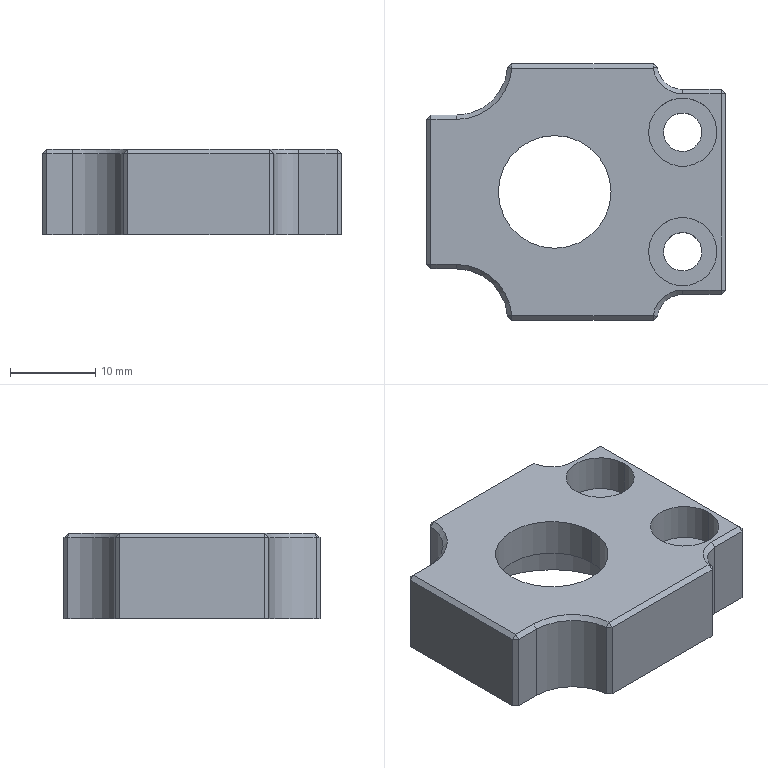Part | STEP file | 03-35 guide bushing mounting seat | 1 solid | 57 faces | box 35 x 30 x 10 mm | volume 5722 mm3 | plane 37 | cylinder 16 | cone 4 | commonest cylinder face diameters 4.5 x4 8 x4 6 x2 12 x2 13.2 x2 22 x2
STEP:
#1=CARTESIAN_POINT('',(8.5,7.,5.6));
#2=VERTEX_POINT('',#1);
#3=CARTESIAN_POINT('',(16.5,7.,5.6));
#4=VERTEX_POINT('',#3);
#5=CARTESIAN_POINT('',(12.5,7.,5.6));
#6=DIRECTION('',(0.,0.,1.));
#7=DIRECTION('',(1.,0.,0.));
#8=AXIS2_PLACEMENT_3D('',#5,#6,#7);
#9=CIRCLE('',#8,4.);
#10=EDGE_CURVE('',#2,#4,#9,.T.);
#11=ORIENTED_EDGE('',*,*,#10,.F.);
#12=CARTESIAN_POINT('',(8.5,7.,10.));
#13=VERTEX_POINT('',#12);
#14=CARTESIAN_POINT('',(8.5,7.,10.));
#15=DIRECTION('',(0.,0.,1.));
#16=VECTOR('',#15,1000.);
#17=LINE('',#14,#16);
#18=EDGE_CURVE('',#2,#13,#17,.T.);
#19=ORIENTED_EDGE('',*,*,#18,.T.);
#20=CARTESIAN_POINT('',(16.5,7.,10.));
#21=VERTEX_POINT('',#20);
#22=CARTESIAN_POINT('',(12.5,7.,10.));
#23=DIRECTION('',(0.,0.,1.));
#24=DIRECTION('',(1.,0.,0.));
#25=AXIS2_PLACEMENT_3D('',#22,#23,#24);
#26=CIRCLE('',#25,4.);
#27=EDGE_CURVE('',#13,#21,#26,.T.);
#28=ORIENTED_EDGE('',*,*,#27,.T.);
#29=CARTESIAN_POINT('',(16.5,7.,10.));
#30=DIRECTION('',(0.,0.,1.));
#31=VECTOR('',#30,1000.);
#32=LINE('',#29,#31);
#33=EDGE_CURVE('',#4,#21,#32,.T.);
#34=ORIENTED_EDGE('',*,*,#33,.F.);
#35=EDGE_LOOP('',(#11,#19,#28,#34));
#36=FACE_OUTER_BOUND('',#35,.T.);
#37=CARTESIAN_POINT('',(12.5,7.,10.));
#38=DIRECTION('',(0.,0.,1.));
#39=DIRECTION('',(1.,0.,0.));
#40=AXIS2_PLACEMENT_3D('',#37,#38,#39);
#41=CYLINDRICAL_SURFACE('',#40,4.);
#42=ADVANCED_FACE('',(#36),#41,.F.);
#43=CARTESIAN_POINT('',(10.25,7.,0.));
#44=VERTEX_POINT('',#43);
#45=CARTESIAN_POINT('',(14.75,7.,0.));
#46=VERTEX_POINT('',#45);
#47=CARTESIAN_POINT('',(12.5,7.,0.));
#48=DIRECTION('',(0.,0.,1.));
#49=DIRECTION('',(1.,0.,0.));
#50=AXIS2_PLACEMENT_3D('',#47,#48,#49);
#51=CIRCLE('',#50,2.25);
#52=EDGE_CURVE('',#44,#46,#51,.T.);
#53=ORIENTED_EDGE('',*,*,#52,.F.);
#54=CARTESIAN_POINT('',(10.25,7.,5.6));
#55=VERTEX_POINT('',#54);
#56=CARTESIAN_POINT('',(10.25,7.,10.));
#57=DIRECTION('',(0.,0.,1.));
#58=VECTOR('',#57,1000.);
#59=LINE('',#56,#58);
#60=EDGE_CURVE('',#44,#55,#59,.T.);
#61=ORIENTED_EDGE('',*,*,#60,.T.);
#62=CARTESIAN_POINT('',(14.75,7.,5.6));
#63=VERTEX_POINT('',#62);
#64=CARTESIAN_POINT('',(12.5,7.,5.6));
#65=DIRECTION('',(0.,0.,1.));
#66=DIRECTION('',(1.,0.,0.));
#67=AXIS2_PLACEMENT_3D('',#64,#65,#66);
#68=CIRCLE('',#67,2.25);
#69=EDGE_CURVE('',#55,#63,#68,.T.);
#70=ORIENTED_EDGE('',*,*,#69,.T.);
#71=CARTESIAN_POINT('',(14.75,7.,10.));
#72=DIRECTION('',(0.,0.,1.));
#73=VECTOR('',#72,1000.);
#74=LINE('',#71,#73);
#75=EDGE_CURVE('',#46,#63,#74,.T.);
#76=ORIENTED_EDGE('',*,*,#75,.F.);
#77=EDGE_LOOP('',(#53,#61,#70,#76));
#78=FACE_OUTER_BOUND('',#77,.T.);
#79=CARTESIAN_POINT('',(12.5,7.,10.));
#80=DIRECTION('',(0.,0.,1.));
#81=DIRECTION('',(1.,0.,0.));
#82=AXIS2_PLACEMENT_3D('',#79,#80,#81);
#83=CYLINDRICAL_SURFACE('',#82,2.25);
#84=ADVANCED_FACE('',(#78),#83,.F.);
#85=CARTESIAN_POINT('',(8.5,-7.,5.6));
#86=VERTEX_POINT('',#85);
#87=CARTESIAN_POINT('',(16.5,-7.,5.6));
#88=VERTEX_POINT('',#87);
#89=CARTESIAN_POINT('',(12.5,-7.,5.6));
#90=DIRECTION('',(0.,0.,1.));
#91=DIRECTION('',(1.,0.,0.));
#92=AXIS2_PLACEMENT_3D('',#89,#90,#91);
#93=CIRCLE('',#92,4.);
#94=EDGE_CURVE('',#86,#88,#93,.T.);
#95=ORIENTED_EDGE('',*,*,#94,.F.);
#96=CARTESIAN_POINT('',(8.5,-7.,10.));
#97=VERTEX_POINT('',#96);
#98=CARTESIAN_POINT('',(8.5,-7.,10.));
#99=DIRECTION('',(0.,0.,1.));
#100=VECTOR('',#99,1000.);
#101=LINE('',#98,#100);
#102=EDGE_CURVE('',#86,#97,#101,.T.);
#103=ORIENTED_EDGE('',*,*,#102,.T.);
#104=CARTESIAN_POINT('',(16.5,-7.,10.));
#105=VERTEX_POINT('',#104);
#106=CARTESIAN_POINT('',(12.5,-7.,10.));
#107=DIRECTION('',(0.,0.,1.));
#108=DIRECTION('',(1.,0.,0.));
#109=AXIS2_PLACEMENT_3D('',#106,#107,#108);
#110=CIRCLE('',#109,4.);
#111=EDGE_CURVE('',#97,#105,#110,.T.);
#112=ORIENTED_EDGE('',*,*,#111,.T.);
#113=CARTESIAN_POINT('',(16.5,-7.,10.));
#114=DIRECTION('',(0.,0.,1.));
#115=VECTOR('',#114,1000.);
#116=LINE('',#113,#115);
#117=EDGE_CURVE('',#88,#105,#116,.T.);
#118=ORIENTED_EDGE('',*,*,#117,.F.);
#119=EDGE_LOOP('',(#95,#103,#112,#118));
#120=FACE_OUTER_BOUND('',#119,.T.);
#121=CARTESIAN_POINT('',(12.5,-7.,10.));
#122=DIRECTION('',(0.,0.,1.));
#123=DIRECTION('',(1.,0.,0.));
#124=AXIS2_PLACEMENT_3D('',#121,#122,#123);
#125=CYLINDRICAL_SURFACE('',#124,4.);
#126=ADVANCED_FACE('',(#120),#125,.F.);
#127=CARTESIAN_POINT('',(10.25,-7.,0.));
#128=VERTEX_POINT('',#127);
#129=CARTESIAN_POINT('',(14.75,-7.,0.));
#130=VERTEX_POINT('',#129);
#131=CARTESIAN_POINT('',(12.5,-7.,0.));
#132=DIRECTION('',(0.,0.,1.));
#133=DIRECTION('',(1.,0.,0.));
#134=AXIS2_PLACEMENT_3D('',#131,#132,#133);
#135=CIRCLE('',#134,2.25);
#136=EDGE_CURVE('',#128,#130,#135,.T.);
#137=ORIENTED_EDGE('',*,*,#136,.F.);
#138=CARTESIAN_POINT('',(10.25,-7.,5.6));
#139=VERTEX_POINT('',#138);
#140=CARTESIAN_POINT('',(10.25,-7.,10.));
#141=DIRECTION('',(0.,0.,1.));
#142=VECTOR('',#141,1000.);
#143=LINE('',#140,#142);
#144=EDGE_CURVE('',#128,#139,#143,.T.);
#145=ORIENTED_EDGE('',*,*,#144,.T.);
#146=CARTESIAN_POINT('',(14.75,-7.,5.6));
#147=VERTEX_POINT('',#146);
#148=CARTESIAN_POINT('',(12.5,-7.,5.6));
#149=DIRECTION('',(0.,0.,1.));
#150=DIRECTION('',(1.,0.,0.));
#151=AXIS2_PLACEMENT_3D('',#148,#149,#150);
#152=CIRCLE('',#151,2.25);
#153=EDGE_CURVE('',#139,#147,#152,.T.);
#154=ORIENTED_EDGE('',*,*,#153,.T.);
#155=CARTESIAN_POINT('',(14.75,-7.,10.));
#156=DIRECTION('',(0.,0.,1.));
#157=VECTOR('',#156,1000.);
#158=LINE('',#155,#157);
#159=EDGE_CURVE('',#130,#147,#158,.T.);
#160=ORIENTED_EDGE('',*,*,#159,.F.);
#161=EDGE_LOOP('',(#137,#145,#154,#160));
#162=FACE_OUTER_BOUND('',#161,.T.);
#163=CARTESIAN_POINT('',(12.5,-7.,10.));
#164=DIRECTION('',(0.,0.,1.));
#165=DIRECTION('',(1.,0.,0.));
#166=AXIS2_PLACEMENT_3D('',#163,#164,#165);
#167=CYLINDRICAL_SURFACE('',#166,2.25);
#168=ADVANCED_FACE('',(#162),#167,.F.);
#169=CARTESIAN_POINT('',(8.5,0.,5.5));
#170=VERTEX_POINT('',#169);
#171=CARTESIAN_POINT('',(-13.5,0.,5.5));
#172=VERTEX_POINT('',#171);
#173=CARTESIAN_POINT('',(-2.5,0.,5.5));
#174=DIRECTION('',(0.,0.,-1.));
#175=DIRECTION('',(-1.,0.,0.));
#176=AXIS2_PLACEMENT_3D('',#173,#174,#175);
#177=CIRCLE('',#176,11.);
#178=EDGE_CURVE('',#170,#172,#177,.T.);
#179=ORIENTED_EDGE('',*,*,#178,.F.);
#180=CARTESIAN_POINT('',(8.5,0.,0.));
#181=VERTEX_POINT('',#180);
#182=CARTESIAN_POINT('',(8.5,0.,5.5));
#183=DIRECTION('',(0.,0.,-1.));
#184=VECTOR('',#183,1000.);
#185=LINE('',#182,#184);
#186=EDGE_CURVE('',#170,#181,#185,.T.);
#187=ORIENTED_EDGE('',*,*,#186,.T.);
#188=CARTESIAN_POINT('',(-13.5,0.,0.));
#189=VERTEX_POINT('',#188);
#190=CARTESIAN_POINT('',(-2.5,0.,0.));
#191=DIRECTION('',(0.,0.,-1.));
#192=DIRECTION('',(-1.,0.,0.));
#193=AXIS2_PLACEMENT_3D('',#190,#191,#192);
#194=CIRCLE('',#193,11.);
#195=EDGE_CURVE('',#181,#189,#194,.T.);
#196=ORIENTED_EDGE('',*,*,#195,.T.);
#197=CARTESIAN_POINT('',(-13.5,0.,5.5));
#198=DIRECTION('',(0.,0.,-1.));
#199=VECTOR('',#198,1000.);
#200=LINE('',#197,#199);
#201=EDGE_CURVE('',#172,#189,#200,.T.);
#202=ORIENTED_EDGE('',*,*,#201,.F.);
#203=EDGE_LOOP('',(#179,#187,#196,#202));
#204=FACE_OUTER_BOUND('',#203,.T.);
#205=CARTESIAN_POINT('',(-2.5,0.,5.5));
#206=DIRECTION('',(0.,0.,-1.));
#207=DIRECTION('',(-1.,0.,0.));
#208=AXIS2_PLACEMENT_3D('',#205,#206,#207);
#209=CYLINDRICAL_SURFACE('',#208,11.);
#210=ADVANCED_FACE('',(#204),#209,.F.);
#211=CARTESIAN_POINT('',(-9.1,0.,5.5));
#212=VERTEX_POINT('',#211);
#213=CARTESIAN_POINT('',(4.1,0.,5.5));
#214=VERTEX_POINT('',#213);
#215=CARTESIAN_POINT('',(-2.5,0.,5.5));
#216=DIRECTION('',(0.,0.,1.));
#217=DIRECTION('',(-1.,0.,0.));
#218=AXIS2_PLACEMENT_3D('',#215,#216,#217);
#219=CIRCLE('',#218,6.6);
#220=EDGE_CURVE('',#212,#214,#219,.T.);
#221=ORIENTED_EDGE('',*,*,#220,.F.);
#222=CARTESIAN_POINT('',(-9.1,0.,10.));
#223=VERTEX_POINT('',#222);
#224=CARTESIAN_POINT('',(-9.1,0.,-10.));
#225=DIRECTION('',(0.,0.,1.));
#226=VECTOR('',#225,1000.);
#227=LINE('',#224,#226);
#228=EDGE_CURVE('',#212,#223,#227,.T.);
#229=ORIENTED_EDGE('',*,*,#228,.T.);
#230=CARTESIAN_POINT('',(4.1,0.,10.));
#231=VERTEX_POINT('',#230);
#232=CARTESIAN_POINT('',(-2.5,0.,10.));
#233=DIRECTION('',(0.,0.,1.));
#234=DIRECTION('',(1.,0.,0.));
#235=AXIS2_PLACEMENT_3D('',#232,#233,#234);
#236=CIRCLE('',#235,6.6);
#237=EDGE_CURVE('',#223,#231,#236,.T.);
#238=ORIENTED_EDGE('',*,*,#237,.T.);
#239=CARTESIAN_POINT('',(4.1,0.,-10.));
#240=DIRECTION('',(0.,0.,1.));
#241=VECTOR('',#240,1000.);
#242=LINE('',#239,#241);
#243=EDGE_CURVE('',#214,#231,#242,.T.);
#244=ORIENTED_EDGE('',*,*,#243,.F.);
#245=EDGE_LOOP('',(#221,#229,#238,#244));
#246=FACE_OUTER_BOUND('',#245,.T.);
#247=CARTESIAN_POINT('',(-2.5,0.,-10.));
#248=DIRECTION('',(0.,0.,1.));
#249=DIRECTION('',(1.,0.,0.));
#250=AXIS2_PLACEMENT_3D('',#247,#248,#249);
#251=CYLINDRICAL_SURFACE('',#250,6.6);
#252=ADVANCED_FACE('',(#246),#251,.F.);
#253=ORIENTED_EDGE('',*,*,#228,.F.);
#254=CARTESIAN_POINT('',(-2.5,0.,5.5));
#255=DIRECTION('',(0.,0.,1.));
#256=DIRECTION('',(-1.,0.,0.));
#257=AXIS2_PLACEMENT_3D('',#254,#255,#256);
#258=CIRCLE('',#257,6.6);
#259=EDGE_CURVE('',#214,#212,#258,.T.);
#260=ORIENTED_EDGE('',*,*,#259,.F.);
#261=ORIENTED_EDGE('',*,*,#243,.T.);
#262=CARTESIAN_POINT('',(-2.5,0.,10.));
#263=DIRECTION('',(0.,0.,1.));
#264=DIRECTION('',(1.,0.,0.));
#265=AXIS2_PLACEMENT_3D('',#262,#263,#264);
#266=CIRCLE('',#265,6.6);
#267=EDGE_CURVE('',#231,#223,#266,.T.);
#268=ORIENTED_EDGE('',*,*,#267,.T.);
#269=EDGE_LOOP('',(#253,#260,#261,#268));
#270=FACE_OUTER_BOUND('',#269,.T.);
#271=CARTESIAN_POINT('',(-2.5,0.,-10.));
#272=DIRECTION('',(0.,0.,1.));
#273=DIRECTION('',(1.,0.,0.));
#274=AXIS2_PLACEMENT_3D('',#271,#272,#273);
#275=CYLINDRICAL_SURFACE('',#274,6.6);
#276=ADVANCED_FACE('',(#270),#275,.F.);
#277=CARTESIAN_POINT('',(17.5,11.5,9.5));
#278=VERTEX_POINT('',#277);
#279=CARTESIAN_POINT('',(17.5,-11.5,9.5));
#280=VERTEX_POINT('',#279);
#281=CARTESIAN_POINT('',(17.5,-12.,9.5));
#282=DIRECTION('',(0.,-1.,0.));
#283=VECTOR('',#282,1000.);
#284=LINE('',#281,#283);
#285=EDGE_CURVE('',#278,#280,#284,.T.);
#286=ORIENTED_EDGE('',*,*,#285,.T.);
#287=CARTESIAN_POINT('',(17.5,-11.5,0.));
#288=VERTEX_POINT('',#287);
#289=CARTESIAN_POINT('',(17.5,-11.5,10.));
#290=DIRECTION('',(0.,0.,-1.));
#291=VECTOR('',#290,1000.);
#292=LINE('',#289,#291);
#293=EDGE_CURVE('',#280,#288,#292,.T.);
#294=ORIENTED_EDGE('',*,*,#293,.T.);
#295=CARTESIAN_POINT('',(17.5,11.5,0.));
#296=VERTEX_POINT('',#295);
#297=CARTESIAN_POINT('',(17.5,15.,0.));
#298=DIRECTION('',(0.,1.,0.));
#299=VECTOR('',#298,1000.);
#300=LINE('',#297,#299);
#301=EDGE_CURVE('',#288,#296,#300,.T.);
#302=ORIENTED_EDGE('',*,*,#301,.T.);
#303=CARTESIAN_POINT('',(17.5,11.5,10.));
#304=DIRECTION('',(0.,0.,1.));
#305=VECTOR('',#304,1000.);
#306=LINE('',#303,#305);
#307=EDGE_CURVE('',#296,#278,#306,.T.);
#308=ORIENTED_EDGE('',*,*,#307,.T.);
#309=EDGE_LOOP('',(#286,#294,#302,#308));
#310=FACE_OUTER_BOUND('',#309,.T.);
#311=CARTESIAN_POINT('',(17.5,15.,10.));
#312=DIRECTION('',(-1.,0.,0.));
#313=DIRECTION('',(0.,-1.,0.));
#314=AXIS2_PLACEMENT_3D('',#311,#312,#313);
#315=PLANE('',#314);
#316=ADVANCED_FACE('',(#310),#315,.F.);
#317=CARTESIAN_POINT('',(-7.519,15.,9.5));
#318=VERTEX_POINT('',#317);
#319=CARTESIAN_POINT('',(9.036,15.,9.5));
#320=VERTEX_POINT('',#319);
#321=CARTESIAN_POINT('',(9.5,15.,9.5));
#322=DIRECTION('',(1.,0.,0.));
#323=VECTOR('',#322,1000.);
#324=LINE('',#321,#323);
#325=EDGE_CURVE('',#318,#320,#324,.T.);
#326=ORIENTED_EDGE('',*,*,#325,.T.);
#327=CARTESIAN_POINT('',(9.036,15.,0.));
#328=VERTEX_POINT('',#327);
#329=CARTESIAN_POINT('',(9.036,15.,10.));
#330=DIRECTION('',(0.,0.,-1.));
#331=VECTOR('',#330,1000.);
#332=LINE('',#329,#331);
#333=EDGE_CURVE('',#320,#328,#332,.T.);
#334=ORIENTED_EDGE('',*,*,#333,.T.);
#335=CARTESIAN_POINT('',(-7.519,15.,0.));
#336=VERTEX_POINT('',#335);
#337=CARTESIAN_POINT('',(-17.5,15.,0.));
#338=DIRECTION('',(-1.,0.,0.));
#339=VECTOR('',#338,1000.);
#340=LINE('',#337,#339);
#341=EDGE_CURVE('',#328,#336,#340,.T.);
#342=ORIENTED_EDGE('',*,*,#341,.T.);
#343=CARTESIAN_POINT('',(-7.519,15.,10.));
#344=DIRECTION('',(0.,0.,1.));
#345=VECTOR('',#344,1000.);
#346=LINE('',#343,#345);
#347=EDGE_CURVE('',#336,#318,#346,.T.);
#348=ORIENTED_EDGE('',*,*,#347,.T.);
#349=EDGE_LOOP('',(#326,#334,#342,#348));
#350=FACE_OUTER_BOUND('',#349,.T.);
#351=CARTESIAN_POINT('',(-17.5,15.,10.));
#352=DIRECTION('',(0.,-1.,0.));
#353=DIRECTION('',(0.,0.,-1.));
#354=AXIS2_PLACEMENT_3D('',#351,#352,#353);
#355=PLANE('',#354);
#356=ADVANCED_FACE('',(#350),#355,.F.);
#357=CARTESIAN_POINT('',(-17.5,-8.5,9.5));
#358=VERTEX_POINT('',#357);
#359=CARTESIAN_POINT('',(-17.5,8.5,9.5));
#360=VERTEX_POINT('',#359);
#361=CARTESIAN_POINT('',(-17.5,9.,9.5));
#362=DIRECTION('',(0.,1.,0.));
#363=VECTOR('',#362,1000.);
#364=LINE('',#361,#363);
#365=EDGE_CURVE('',#358,#360,#364,.T.);
#366=ORIENTED_EDGE('',*,*,#365,.T.);
#367=CARTESIAN_POINT('',(-17.5,8.5,0.));
#368=VERTEX_POINT('',#367);
#369=CARTESIAN_POINT('',(-17.5,8.5,10.));
#370=DIRECTION('',(0.,0.,-1.));
#371=VECTOR('',#370,1000.);
#372=LINE('',#369,#371);
#373=EDGE_CURVE('',#360,#368,#372,.T.);
#374=ORIENTED_EDGE('',*,*,#373,.T.);
#375=CARTESIAN_POINT('',(-17.5,-8.5,0.));
#376=VERTEX_POINT('',#375);
#377=CARTESIAN_POINT('',(-17.5,15.,0.));
#378=DIRECTION('',(0.,-1.,0.));
#379=VECTOR('',#378,1000.);
#380=LINE('',#377,#379);
#381=EDGE_CURVE('',#368,#376,#380,.T.);
#382=ORIENTED_EDGE('',*,*,#381,.T.);
#383=CARTESIAN_POINT('',(-17.5,-8.5,10.));
#384=DIRECTION('',(0.,0.,1.));
#385=VECTOR('',#384,1000.);
#386=LINE('',#383,#385);
#387=EDGE_CURVE('',#376,#358,#386,.T.);
#388=ORIENTED_EDGE('',*,*,#387,.T.);
#389=EDGE_LOOP('',(#366,#374,#382,#388));
#390=FACE_OUTER_BOUND('',#389,.T.);
#391=CARTESIAN_POINT('',(-17.5,15.,10.));
#392=DIRECTION('',(1.,0.,0.));
#393=DIRECTION('',(0.,1.,0.));
#394=AXIS2_PLACEMENT_3D('',#391,#392,#393);
#395=PLANE('',#394);
#396=ADVANCED_FACE('',(#390),#395,.F.);
#397=CARTESIAN_POINT('',(9.036,-15.,9.5));
#398=VERTEX_POINT('',#397);
#399=CARTESIAN_POINT('',(-7.519,-15.,9.5));
#400=VERTEX_POINT('',#399);
#401=CARTESIAN_POINT('',(-8.,-15.,9.5));
#402=DIRECTION('',(-1.,0.,0.));
#403=VECTOR('',#402,1000.);
#404=LINE('',#401,#403);
#405=EDGE_CURVE('',#398,#400,#404,.T.);
#406=ORIENTED_EDGE('',*,*,#405,.T.);
#407=CARTESIAN_POINT('',(-7.519,-15.,0.));
#408=VERTEX_POINT('',#407);
#409=CARTESIAN_POINT('',(-7.519,-15.,10.));
#410=DIRECTION('',(0.,0.,-1.));
#411=VECTOR('',#410,1000.);
#412=LINE('',#409,#411);
#413=EDGE_CURVE('',#400,#408,#412,.T.);
#414=ORIENTED_EDGE('',*,*,#413,.T.);
#415=CARTESIAN_POINT('',(9.036,-15.,0.));
#416=VERTEX_POINT('',#415);
#417=CARTESIAN_POINT('',(-17.5,-15.,0.));
#418=DIRECTION('',(1.,0.,0.));
#419=VECTOR('',#418,1000.);
#420=LINE('',#417,#419);
#421=EDGE_CURVE('',#408,#416,#420,.T.);
#422=ORIENTED_EDGE('',*,*,#421,.T.);
#423=CARTESIAN_POINT('',(9.036,-15.,10.));
#424=DIRECTION('',(0.,0.,1.));
#425=VECTOR('',#424,1000.);
#426=LINE('',#423,#425);
#427=EDGE_CURVE('',#416,#398,#426,.T.);
#428=ORIENTED_EDGE('',*,*,#427,.T.);
#429=EDGE_LOOP('',(#406,#414,#422,#428));
#430=FACE_OUTER_BOUND('',#429,.T.);
#431=CARTESIAN_POINT('',(-17.5,-15.,10.));
#432=DIRECTION('',(0.,1.,0.));
#433=DIRECTION('',(0.,0.,1.));
#434=AXIS2_PLACEMENT_3D('',#431,#432,#433);
#435=PLANE('',#434);
#436=ADVANCED_FACE('',(#430),#435,.F.);
#437=CARTESIAN_POINT('',(12.5,-11.5,10.));
#438=VERTEX_POINT('',#437);
#439=CARTESIAN_POINT('',(17.,-11.5,10.));
#440=VERTEX_POINT('',#439);
#441=CARTESIAN_POINT('',(17.5,-11.5,10.));
#442=DIRECTION('',(1.,0.,0.));
#443=VECTOR('',#442,1000.);
#444=LINE('',#441,#443);
#445=EDGE_CURVE('',#438,#440,#444,.T.);
#446=ORIENTED_EDGE('',*,*,#445,.T.);
#447=CARTESIAN_POINT('',(17.,11.5,10.));
#448=VERTEX_POINT('',#447);
#449=CARTESIAN_POINT('',(17.,12.,10.));
#450=DIRECTION('',(0.,1.,0.));
#451=VECTOR('',#450,1000.);
#452=LINE('',#449,#451);
#453=EDGE_CURVE('',#440,#448,#452,.T.);
#454=ORIENTED_EDGE('',*,*,#453,.T.);
#455=CARTESIAN_POINT('',(12.5,11.5,10.));
#456=VERTEX_POINT('',#455);
#457=CARTESIAN_POINT('',(12.5,11.5,10.));
#458=DIRECTION('',(-1.,0.,0.));
#459=VECTOR('',#458,1000.);
#460=LINE('',#457,#459);
#461=EDGE_CURVE('',#448,#456,#460,.T.);
#462=ORIENTED_EDGE('',*,*,#461,.T.);
#463=CARTESIAN_POINT('',(9.036,14.5,10.));
#464=VERTEX_POINT('',#463);
#465=CARTESIAN_POINT('',(12.5,15.,10.));
#466=DIRECTION('',(0.,0.,-1.));
#467=DIRECTION('',(1.,0.,0.));
#468=AXIS2_PLACEMENT_3D('',#465,#466,#467);
#469=CIRCLE('',#468,3.5);
#470=EDGE_CURVE('',#456,#464,#469,.T.);
#471=ORIENTED_EDGE('',*,*,#470,.T.);
#472=CARTESIAN_POINT('',(-7.519,14.5,10.));
#473=VERTEX_POINT('',#472);
#474=CARTESIAN_POINT('',(-8.,14.5,10.));
#475=DIRECTION('',(-1.,0.,0.));
#476=VECTOR('',#475,1000.);
#477=LINE('',#474,#476);
#478=EDGE_CURVE('',#464,#473,#477,.T.);
#479=ORIENTED_EDGE('',*,*,#478,.T.);
#480=CARTESIAN_POINT('',(-14.,8.5,10.));
#481=VERTEX_POINT('',#480);
#482=CARTESIAN_POINT('',(-14.,15.,10.));
#483=DIRECTION('',(0.,0.,-1.));
#484=DIRECTION('',(1.,0.,0.));
#485=AXIS2_PLACEMENT_3D('',#482,#483,#484);
#486=CIRCLE('',#485,6.5);
#487=EDGE_CURVE('',#473,#481,#486,.T.);
#488=ORIENTED_EDGE('',*,*,#487,.T.);
#489=CARTESIAN_POINT('',(-17.,8.5,10.));
#490=VERTEX_POINT('',#489);
#491=CARTESIAN_POINT('',(-17.5,8.5,10.));
#492=DIRECTION('',(-1.,0.,0.));
#493=VECTOR('',#492,1000.);
#494=LINE('',#491,#493);
#495=EDGE_CURVE('',#481,#490,#494,.T.);
#496=ORIENTED_EDGE('',*,*,#495,.T.);
#497=CARTESIAN_POINT('',(-17.,-8.5,10.));
#498=VERTEX_POINT('',#497);
#499=CARTESIAN_POINT('',(-17.,-9.,10.));
#500=DIRECTION('',(0.,-1.,0.));
#501=VECTOR('',#500,1000.);
#502=LINE('',#499,#501);
#503=EDGE_CURVE('',#490,#498,#502,.T.);
#504=ORIENTED_EDGE('',*,*,#503,.T.);
#505=CARTESIAN_POINT('',(-14.,-8.5,10.));
#506=VERTEX_POINT('',#505);
#507=CARTESIAN_POINT('',(-14.,-8.5,10.));
#508=DIRECTION('',(1.,0.,0.));
#509=VECTOR('',#508,1000.);
#510=LINE('',#507,#509);
#511=EDGE_CURVE('',#498,#506,#510,.T.);
#512=ORIENTED_EDGE('',*,*,#511,.T.);
#513=CARTESIAN_POINT('',(-7.519,-14.5,10.));
#514=VERTEX_POINT('',#513);
#515=CARTESIAN_POINT('',(-14.,-15.,10.));
#516=DIRECTION('',(0.,0.,-1.));
#517=DIRECTION('',(1.,0.,0.));
#518=AXIS2_PLACEMENT_3D('',#515,#516,#517);
#519=CIRCLE('',#518,6.5);
#520=EDGE_CURVE('',#506,#514,#519,.T.);
#521=ORIENTED_EDGE('',*,*,#520,.T.);
#522=CARTESIAN_POINT('',(9.036,-14.5,10.));
#523=VERTEX_POINT('',#522);
#524=CARTESIAN_POINT('',(9.5,-14.5,10.));
#525=DIRECTION('',(1.,0.,0.));
#526=VECTOR('',#525,1000.);
#527=LINE('',#524,#526);
#528=EDGE_CURVE('',#514,#523,#527,.T.);
#529=ORIENTED_EDGE('',*,*,#528,.T.);
#530=CARTESIAN_POINT('',(12.5,-15.,10.));
#531=DIRECTION('',(0.,0.,-1.));
#532=DIRECTION('',(1.,0.,0.));
#533=AXIS2_PLACEMENT_3D('',#530,#531,#532);
#534=CIRCLE('',#533,3.5);
#535=EDGE_CURVE('',#523,#438,#534,.T.);
#536=ORIENTED_EDGE('',*,*,#535,.T.);
#537=EDGE_LOOP('',(#446,#454,#462,#471,#479,#488,#496,#504,#512,#521,#529,#536));
#538=FACE_OUTER_BOUND('',#537,.T.);
#539=CARTESIAN_POINT('',(12.5,7.,10.));
#540=DIRECTION('',(0.,0.,1.));
#541=DIRECTION('',(1.,0.,0.));
#542=AXIS2_PLACEMENT_3D('',#539,#540,#541);
#543=CIRCLE('',#542,4.);
#544=EDGE_CURVE('',#21,#13,#543,.T.);
#545=ORIENTED_EDGE('',*,*,#544,.F.);
#546=ORIENTED_EDGE('',*,*,#27,.F.);
#547=EDGE_LOOP('',(#545,#546));
#548=FACE_BOUND('',#547,.T.);
#549=CARTESIAN_POINT('',(12.5,-7.,10.));
#550=DIRECTION('',(0.,0.,1.));
#551=DIRECTION('',(1.,0.,0.));
#552=AXIS2_PLACEMENT_3D('',#549,#550,#551);
#553=CIRCLE('',#552,4.);
#554=EDGE_CURVE('',#105,#97,#553,.T.);
#555=ORIENTED_EDGE('',*,*,#554,.F.);
#556=ORIENTED_EDGE('',*,*,#111,.F.);
#557=EDGE_LOOP('',(#555,#556));
#558=FACE_BOUND('',#557,.T.);
#559=ORIENTED_EDGE('',*,*,#267,.F.);
#560=ORIENTED_EDGE('',*,*,#237,.F.);
#561=EDGE_LOOP('',(#559,#560));
#562=FACE_BOUND('',#561,.T.);
#563=CARTESIAN_POINT('',(17.5,-15.,10.));
#564=DIRECTION('',(0.,0.,1.));
#565=DIRECTION('',(1.,0.,0.));
#566=AXIS2_PLACEMENT_3D('',#563,#564,#565);
#567=PLANE('',#566);
#568=ADVANCED_FACE('',(#538,#548,#558,#562),#567,.T.);
#569=CARTESIAN_POINT('',(12.5,7.,0.));
#570=DIRECTION('',(0.,0.,1.));
#571=DIRECTION('',(1.,0.,0.));
#572=AXIS2_PLACEMENT_3D('',#569,#570,#571);
#573=CIRCLE('',#572,2.25);
#574=EDGE_CURVE('',#46,#44,#573,.T.);
#575=ORIENTED_EDGE('',*,*,#574,.T.);
#576=ORIENTED_EDGE('',*,*,#52,.T.);
#577=EDGE_LOOP('',(#575,#576));
#578=FACE_BOUND('',#577,.T.);
#579=CARTESIAN_POINT('',(12.5,-7.,0.));
#580=DIRECTION('',(0.,0.,1.));
#581=DIRECTION('',(1.,0.,0.));
#582=AXIS2_PLACEMENT_3D('',#579,#580,#581);
#583=CIRCLE('',#582,2.25);
#584=EDGE_CURVE('',#130,#128,#583,.T.);
#585=ORIENTED_EDGE('',*,*,#584,.T.);
#586=ORIENTED_EDGE('',*,*,#136,.T.);
#587=EDGE_LOOP('',(#585,#586));
#588=FACE_BOUND('',#587,.T.);
#589=CARTESIAN_POINT('',(-2.5,0.,0.));
#590=DIRECTION('',(0.,0.,-1.));
#591=DIRECTION('',(-1.,0.,0.));
#592=AXIS2_PLACEMENT_3D('',#589,#590,#591);
#593=CIRCLE('',#592,11.);
#594=EDGE_CURVE('',#189,#181,#593,.T.);
#595=ORIENTED_EDGE('',*,*,#594,.F.);
#596=ORIENTED_EDGE('',*,*,#195,.F.);
#597=EDGE_LOOP('',(#595,#596));
#598=FACE_BOUND('',#597,.T.);
#599=ORIENTED_EDGE('',*,*,#301,.F.);
#600=CARTESIAN_POINT('',(17.,-12.,0.));
#601=VERTEX_POINT('',#600);
#602=CARTESIAN_POINT('',(17.,-12.,0.));
#603=DIRECTION('',(-0.7071,-0.7071,0.));
#604=VECTOR('',#603,1000.);
#605=LINE('',#602,#604);
#606=EDGE_CURVE('',#288,#601,#605,.T.);
#607=ORIENTED_EDGE('',*,*,#606,.T.);
#608=CARTESIAN_POINT('',(12.5,-12.,0.));
#609=VERTEX_POINT('',#608);
#610=CARTESIAN_POINT('',(17.5,-12.,0.));
#611=DIRECTION('',(-1.,0.,0.));
#612=VECTOR('',#611,1000.);
#613=LINE('',#610,#612);
#614=EDGE_CURVE('',#601,#609,#613,.T.);
#615=ORIENTED_EDGE('',*,*,#614,.T.);
#616=CARTESIAN_POINT('',(9.531,-14.571,0.));
#617=VERTEX_POINT('',#616);
#618=CARTESIAN_POINT('',(12.5,-15.,0.));
#619=DIRECTION('',(0.,0.,1.));
#620=DIRECTION('',(1.,0.,0.));
#621=AXIS2_PLACEMENT_3D('',#618,#619,#620);
#622=CIRCLE('',#621,3.);
#623=EDGE_CURVE('',#609,#617,#622,.T.);
#624=ORIENTED_EDGE('',*,*,#623,.T.);
#625=CARTESIAN_POINT('',(9.036,-15.,0.));
#626=DIRECTION('',(-0.7559,-0.6547,0.));
#627=VECTOR('',#626,1000.);
#628=LINE('',#625,#627);
#629=EDGE_CURVE('',#617,#416,#628,.T.);
#630=ORIENTED_EDGE('',*,*,#629,.T.);
#631=ORIENTED_EDGE('',*,*,#421,.F.);
#632=CARTESIAN_POINT('',(-8.018,-14.538,0.));
#633=VERTEX_POINT('',#632);
#634=CARTESIAN_POINT('',(-8.018,-14.538,0.));
#635=DIRECTION('',(-0.7338,0.6794,0.));
#636=VECTOR('',#635,1000.);
#637=LINE('',#634,#636);
#638=EDGE_CURVE('',#408,#633,#637,.T.);
#639=ORIENTED_EDGE('',*,*,#638,.T.);
#640=CARTESIAN_POINT('',(-14.,-9.,0.));
#641=VERTEX_POINT('',#640);
#642=CARTESIAN_POINT('',(-14.,-15.,0.));
#643=DIRECTION('',(0.,0.,1.));
#644=DIRECTION('',(1.,0.,0.));
#645=AXIS2_PLACEMENT_3D('',#642,#643,#644);
#646=CIRCLE('',#645,6.);
#647=EDGE_CURVE('',#633,#641,#646,.T.);
#648=ORIENTED_EDGE('',*,*,#647,.T.);
#649=CARTESIAN_POINT('',(-17.,-9.,0.));
#650=VERTEX_POINT('',#649);
#651=CARTESIAN_POINT('',(17.5,-9.,0.));
#652=DIRECTION('',(-1.,0.,0.));
#653=VECTOR('',#652,1000.);
#654=LINE('',#651,#653);
#655=EDGE_CURVE('',#641,#650,#654,.T.);
#656=ORIENTED_EDGE('',*,*,#655,.T.);
#657=CARTESIAN_POINT('',(-17.5,-8.5,0.));
#658=DIRECTION('',(-0.7071,0.7071,0.));
#659=VECTOR('',#658,1000.);
#660=LINE('',#657,#659);
#661=EDGE_CURVE('',#650,#376,#660,.T.);
#662=ORIENTED_EDGE('',*,*,#661,.T.);
#663=ORIENTED_EDGE('',*,*,#381,.F.);
#664=CARTESIAN_POINT('',(-17.,9.,0.));
#665=VERTEX_POINT('',#664);
#666=CARTESIAN_POINT('',(-17.5,8.5,0.));
#667=DIRECTION('',(0.7071,0.7071,0.));
#668=VECTOR('',#667,1000.);
#669=LINE('',#666,#668);
#670=EDGE_CURVE('',#368,#665,#669,.T.);
#671=ORIENTED_EDGE('',*,*,#670,.T.);
#672=CARTESIAN_POINT('',(-14.,9.,0.));
#673=VERTEX_POINT('',#672);
#674=CARTESIAN_POINT('',(17.5,9.,0.));
#675=DIRECTION('',(1.,0.,0.));
#676=VECTOR('',#675,1000.);
#677=LINE('',#674,#676);
#678=EDGE_CURVE('',#665,#673,#677,.T.);
#679=ORIENTED_EDGE('',*,*,#678,.T.);
#680=CARTESIAN_POINT('',(-8.018,14.538,0.));
#681=VERTEX_POINT('',#680);
#682=CARTESIAN_POINT('',(-14.,15.,0.));
#683=DIRECTION('',(0.,0.,1.));
#684=DIRECTION('',(1.,0.,0.));
#685=AXIS2_PLACEMENT_3D('',#682,#683,#684);
#686=CIRCLE('',#685,6.);
#687=EDGE_CURVE('',#673,#681,#686,.T.);
#688=ORIENTED_EDGE('',*,*,#687,.T.);
#689=CARTESIAN_POINT('',(-7.519,15.,0.));
#690=DIRECTION('',(0.7338,0.6794,0.));
#691=VECTOR('',#690,1000.);
#692=LINE('',#689,#691);
#693=EDGE_CURVE('',#681,#336,#692,.T.);
#694=ORIENTED_EDGE('',*,*,#693,.T.);
#695=ORIENTED_EDGE('',*,*,#341,.F.);
#696=CARTESIAN_POINT('',(9.531,14.571,0.));
#697=VERTEX_POINT('',#696);
#698=CARTESIAN_POINT('',(9.531,14.571,0.));
#699=DIRECTION('',(0.7559,-0.6547,0.));
#700=VECTOR('',#699,1000.);
#701=LINE('',#698,#700);
#702=EDGE_CURVE('',#328,#697,#701,.T.);
#703=ORIENTED_EDGE('',*,*,#702,.T.);
#704=CARTESIAN_POINT('',(12.5,12.,0.));
#705=VERTEX_POINT('',#704);
#706=CARTESIAN_POINT('',(12.5,15.,0.));
#707=DIRECTION('',(0.,0.,1.));
#708=DIRECTION('',(1.,0.,0.));
#709=AXIS2_PLACEMENT_3D('',#706,#707,#708);
#710=CIRCLE('',#709,3.);
#711=EDGE_CURVE('',#697,#705,#710,.T.);
#712=ORIENTED_EDGE('',*,*,#711,.T.);
#713=CARTESIAN_POINT('',(17.,12.,0.));
#714=VERTEX_POINT('',#713);
#715=CARTESIAN_POINT('',(17.5,12.,0.));
#716=DIRECTION('',(1.,0.,0.));
#717=VECTOR('',#716,1000.);
#718=LINE('',#715,#717);
#719=EDGE_CURVE('',#705,#714,#718,.T.);
#720=ORIENTED_EDGE('',*,*,#719,.T.);
#721=CARTESIAN_POINT('',(17.5,11.5,0.));
#722=DIRECTION('',(0.7071,-0.7071,0.));
#723=VECTOR('',#722,1000.);
#724=LINE('',#721,#723);
#725=EDGE_CURVE('',#714,#296,#724,.T.);
#726=ORIENTED_EDGE('',*,*,#725,.T.);
#727=EDGE_LOOP('',(#599,#607,#615,#624,#630,#631,#639,#648,#656,#662,#663,#671,#679,#688,#694,#695,#703,#712,#720,#726));
#728=FACE_OUTER_BOUND('',#727,.T.);
#729=CARTESIAN_POINT('',(17.5,-15.,0.));
#730=DIRECTION('',(0.,0.,1.));
#731=DIRECTION('',(1.,0.,0.));
#732=AXIS2_PLACEMENT_3D('',#729,#730,#731);
#733=PLANE('',#732);
#734=ADVANCED_FACE('',(#578,#588,#598,#728),#733,.F.);
#735=CARTESIAN_POINT('',(-14.,-9.,9.5));
#736=VERTEX_POINT('',#735);
#737=CARTESIAN_POINT('',(-17.,-9.,9.5));
#738=VERTEX_POINT('',#737);
#739=CARTESIAN_POINT('',(-17.5,-9.,9.5));
#740=DIRECTION('',(-1.,0.,0.));
#741=VECTOR('',#740,1000.);
#742=LINE('',#739,#741);
#743=EDGE_CURVE('',#736,#738,#742,.T.);
#744=ORIENTED_EDGE('',*,*,#743,.T.);
#745=CARTESIAN_POINT('',(-17.,-9.,-10.));
#746=DIRECTION('',(0.,0.,-1.));
#747=VECTOR('',#746,1000.);
#748=LINE('',#745,#747);
#749=EDGE_CURVE('',#738,#650,#748,.T.);
#750=ORIENTED_EDGE('',*,*,#749,.T.);
#751=ORIENTED_EDGE('',*,*,#655,.F.);
#752=CARTESIAN_POINT('',(-14.,-9.,10.));
#753=DIRECTION('',(0.,0.,1.));
#754=VECTOR('',#753,1000.);
#755=LINE('',#752,#754);
#756=EDGE_CURVE('',#641,#736,#755,.T.);
#757=ORIENTED_EDGE('',*,*,#756,.T.);
#758=EDGE_LOOP('',(#744,#750,#751,#757));
#759=FACE_OUTER_BOUND('',#758,.T.);
#760=CARTESIAN_POINT('',(-20.,-9.,-10.));
#761=DIRECTION('',(0.,1.,0.));
#762=DIRECTION('',(0.,0.,1.));
#763=AXIS2_PLACEMENT_3D('',#760,#761,#762);
#764=PLANE('',#763);
#765=ADVANCED_FACE('',(#759),#764,.F.);
#766=CARTESIAN_POINT('',(-17.,9.,9.5));
#767=VERTEX_POINT('',#766);
#768=CARTESIAN_POINT('',(-17.,9.,-10.));
#769=DIRECTION('',(0.,0.,1.));
#770=VECTOR('',#769,1000.);
#771=LINE('',#768,#770);
#772=EDGE_CURVE('',#665,#767,#771,.T.);
#773=ORIENTED_EDGE('',*,*,#772,.T.);
#774=CARTESIAN_POINT('',(-14.,9.,9.5));
#775=VERTEX_POINT('',#774);
#776=CARTESIAN_POINT('',(-14.,9.,9.5));
#777=DIRECTION('',(1.,0.,0.));
#778=VECTOR('',#777,1000.);
#779=LINE('',#776,#778);
#780=EDGE_CURVE('',#767,#775,#779,.T.);
#781=ORIENTED_EDGE('',*,*,#780,.T.);
#782=CARTESIAN_POINT('',(-14.,9.,5.5));
#783=DIRECTION('',(0.,0.,-1.));
#784=VECTOR('',#783,1000.);
#785=LINE('',#782,#784);
#786=EDGE_CURVE('',#775,#673,#785,.T.);
#787=ORIENTED_EDGE('',*,*,#786,.T.);
#788=ORIENTED_EDGE('',*,*,#678,.F.);
#789=EDGE_LOOP('',(#773,#781,#787,#788));
#790=FACE_OUTER_BOUND('',#789,.T.);
#791=CARTESIAN_POINT('',(-20.,9.,-10.));
#792=DIRECTION('',(0.,-1.,0.));
#793=DIRECTION('',(0.,0.,-1.));
#794=AXIS2_PLACEMENT_3D('',#791,#792,#793);
#795=PLANE('',#794);
#796=ADVANCED_FACE('',(#790),#795,.F.);
#797=ORIENTED_EDGE('',*,*,#186,.F.);
#798=CARTESIAN_POINT('',(-2.5,0.,5.5));
#799=DIRECTION('',(0.,0.,-1.));
#800=DIRECTION('',(-1.,0.,0.));
#801=AXIS2_PLACEMENT_3D('',#798,#799,#800);
#802=CIRCLE('',#801,11.);
#803=EDGE_CURVE('',#172,#170,#802,.T.);
#804=ORIENTED_EDGE('',*,*,#803,.F.);
#805=ORIENTED_EDGE('',*,*,#201,.T.);
#806=ORIENTED_EDGE('',*,*,#594,.T.);
#807=EDGE_LOOP('',(#797,#804,#805,#806));
#808=FACE_OUTER_BOUND('',#807,.T.);
#809=CARTESIAN_POINT('',(-2.5,0.,5.5));
#810=DIRECTION('',(0.,0.,-1.));
#811=DIRECTION('',(-1.,0.,0.));
#812=AXIS2_PLACEMENT_3D('',#809,#810,#811);
#813=CYLINDRICAL_SURFACE('',#812,11.);
#814=ADVANCED_FACE('',(#808),#813,.F.);
#815=ORIENTED_EDGE('',*,*,#259,.T.);
#816=ORIENTED_EDGE('',*,*,#220,.T.);
#817=EDGE_LOOP('',(#815,#816));
#818=FACE_BOUND('',#817,.T.);
#819=ORIENTED_EDGE('',*,*,#803,.T.);
#820=ORIENTED_EDGE('',*,*,#178,.T.);
#821=EDGE_LOOP('',(#819,#820));
#822=FACE_OUTER_BOUND('',#821,.T.);
#823=CARTESIAN_POINT('',(-2.5,0.,5.5));
#824=DIRECTION('',(0.,0.,-1.));
#825=DIRECTION('',(-1.,0.,0.));
#826=AXIS2_PLACEMENT_3D('',#823,#824,#825);
#827=PLANE('',#826);
#828=ADVANCED_FACE('',(#818,#822),#827,.T.);
#829=ORIENTED_EDGE('',*,*,#647,.F.);
#830=CARTESIAN_POINT('',(-8.018,-14.538,9.5));
#831=VERTEX_POINT('',#830);
#832=CARTESIAN_POINT('',(-8.018,-14.538,-10.));
#833=DIRECTION('',(0.,0.,1.));
#834=VECTOR('',#833,1000.);
#835=LINE('',#832,#834);
#836=EDGE_CURVE('',#633,#831,#835,.T.);
#837=ORIENTED_EDGE('',*,*,#836,.T.);
#838=CARTESIAN_POINT('',(-14.,-15.,9.5));
#839=DIRECTION('',(0.,0.,1.));
#840=DIRECTION('',(1.,0.,0.));
#841=AXIS2_PLACEMENT_3D('',#838,#839,#840);
#842=CIRCLE('',#841,6.);
#843=EDGE_CURVE('',#831,#736,#842,.T.);
#844=ORIENTED_EDGE('',*,*,#843,.T.);
#845=ORIENTED_EDGE('',*,*,#756,.F.);
#846=EDGE_LOOP('',(#829,#837,#844,#845));
#847=FACE_OUTER_BOUND('',#846,.T.);
#848=CARTESIAN_POINT('',(-14.,-15.,-10.));
#849=DIRECTION('',(0.,0.,-1.));
#850=DIRECTION('',(-1.,0.,0.));
#851=AXIS2_PLACEMENT_3D('',#848,#849,#850);
#852=CYLINDRICAL_SURFACE('',#851,6.);
#853=ADVANCED_FACE('',(#847),#852,.F.);
#854=CARTESIAN_POINT('',(-8.018,14.538,9.5));
#855=VERTEX_POINT('',#854);
#856=CARTESIAN_POINT('',(-14.,15.,9.5));
#857=DIRECTION('',(0.,0.,1.));
#858=DIRECTION('',(1.,0.,0.));
#859=AXIS2_PLACEMENT_3D('',#856,#857,#858);
#860=CIRCLE('',#859,6.);
#861=EDGE_CURVE('',#775,#855,#860,.T.);
#862=ORIENTED_EDGE('',*,*,#861,.T.);
#863=CARTESIAN_POINT('',(-8.018,14.538,-10.));
#864=DIRECTION('',(0.,0.,-1.));
#865=VECTOR('',#864,1000.);
#866=LINE('',#863,#865);
#867=EDGE_CURVE('',#855,#681,#866,.T.);
#868=ORIENTED_EDGE('',*,*,#867,.T.);
#869=ORIENTED_EDGE('',*,*,#687,.F.);
#870=ORIENTED_EDGE('',*,*,#786,.F.);
#871=EDGE_LOOP('',(#862,#868,#869,#870));
#872=FACE_OUTER_BOUND('',#871,.T.);
#873=CARTESIAN_POINT('',(-14.,15.,-10.));
#874=DIRECTION('',(0.,0.,-1.));
#875=DIRECTION('',(-1.,0.,0.));
#876=AXIS2_PLACEMENT_3D('',#873,#874,#875);
#877=CYLINDRICAL_SURFACE('',#876,6.);
#878=ADVANCED_FACE('',(#872),#877,.F.);
#879=ORIENTED_EDGE('',*,*,#144,.F.);
#880=ORIENTED_EDGE('',*,*,#584,.F.);
#881=ORIENTED_EDGE('',*,*,#159,.T.);
#882=CARTESIAN_POINT('',(12.5,-7.,5.6));
#883=DIRECTION('',(0.,0.,1.));
#884=DIRECTION('',(1.,0.,0.));
#885=AXIS2_PLACEMENT_3D('',#882,#883,#884);
#886=CIRCLE('',#885,2.25);
#887=EDGE_CURVE('',#147,#139,#886,.T.);
#888=ORIENTED_EDGE('',*,*,#887,.T.);
#889=EDGE_LOOP('',(#879,#880,#881,#888));
#890=FACE_OUTER_BOUND('',#889,.T.);
#891=CARTESIAN_POINT('',(12.5,-7.,10.));
#892=DIRECTION('',(0.,0.,1.));
#893=DIRECTION('',(1.,0.,0.));
#894=AXIS2_PLACEMENT_3D('',#891,#892,#893);
#895=CYLINDRICAL_SURFACE('',#894,2.25);
#896=ADVANCED_FACE('',(#890),#895,.F.);
#897=ORIENTED_EDGE('',*,*,#887,.F.);
#898=ORIENTED_EDGE('',*,*,#153,.F.);
#899=EDGE_LOOP('',(#897,#898));
#900=FACE_BOUND('',#899,.T.);
#901=CARTESIAN_POINT('',(12.5,-7.,5.6));
#902=DIRECTION('',(0.,0.,1.));
#903=DIRECTION('',(1.,0.,0.));
#904=AXIS2_PLACEMENT_3D('',#901,#902,#903);
#905=CIRCLE('',#904,4.);
#906=EDGE_CURVE('',#88,#86,#905,.T.);
#907=ORIENTED_EDGE('',*,*,#906,.T.);
#908=ORIENTED_EDGE('',*,*,#94,.T.);
#909=EDGE_LOOP('',(#907,#908));
#910=FACE_OUTER_BOUND('',#909,.T.);
#911=CARTESIAN_POINT('',(14.75,-7.,5.6));
#912=DIRECTION('',(0.,0.,-1.));
#913=DIRECTION('',(-1.,0.,0.));
#914=AXIS2_PLACEMENT_3D('',#911,#912,#913);
#915=PLANE('',#914);
#916=ADVANCED_FACE('',(#900,#910),#915,.F.);
#917=ORIENTED_EDGE('',*,*,#102,.F.);
#918=ORIENTED_EDGE('',*,*,#906,.F.);
#919=ORIENTED_EDGE('',*,*,#117,.T.);
#920=ORIENTED_EDGE('',*,*,#554,.T.);
#921=EDGE_LOOP('',(#917,#918,#919,#920));
#922=FACE_OUTER_BOUND('',#921,.T.);
#923=CARTESIAN_POINT('',(12.5,-7.,10.));
#924=DIRECTION('',(0.,0.,1.));
#925=DIRECTION('',(1.,0.,0.));
#926=AXIS2_PLACEMENT_3D('',#923,#924,#925);
#927=CYLINDRICAL_SURFACE('',#926,4.);
#928=ADVANCED_FACE('',(#922),#927,.F.);
#929=ORIENTED_EDGE('',*,*,#60,.F.);
#930=ORIENTED_EDGE('',*,*,#574,.F.);
#931=ORIENTED_EDGE('',*,*,#75,.T.);
#932=CARTESIAN_POINT('',(12.5,7.,5.6));
#933=DIRECTION('',(0.,0.,1.));
#934=DIRECTION('',(1.,0.,0.));
#935=AXIS2_PLACEMENT_3D('',#932,#933,#934);
#936=CIRCLE('',#935,2.25);
#937=EDGE_CURVE('',#63,#55,#936,.T.);
#938=ORIENTED_EDGE('',*,*,#937,.T.);
#939=EDGE_LOOP('',(#929,#930,#931,#938));
#940=FACE_OUTER_BOUND('',#939,.T.);
#941=CARTESIAN_POINT('',(12.5,7.,10.));
#942=DIRECTION('',(0.,0.,1.));
#943=DIRECTION('',(1.,0.,0.));
#944=AXIS2_PLACEMENT_3D('',#941,#942,#943);
#945=CYLINDRICAL_SURFACE('',#944,2.25);
#946=ADVANCED_FACE('',(#940),#945,.F.);
#947=ORIENTED_EDGE('',*,*,#937,.F.);
#948=ORIENTED_EDGE('',*,*,#69,.F.);
#949=EDGE_LOOP('',(#947,#948));
#950=FACE_BOUND('',#949,.T.);
#951=CARTESIAN_POINT('',(12.5,7.,5.6));
#952=DIRECTION('',(0.,0.,1.));
#953=DIRECTION('',(1.,0.,0.));
#954=AXIS2_PLACEMENT_3D('',#951,#952,#953);
#955=CIRCLE('',#954,4.);
#956=EDGE_CURVE('',#4,#2,#955,.T.);
#957=ORIENTED_EDGE('',*,*,#956,.T.);
#958=ORIENTED_EDGE('',*,*,#10,.T.);
#959=EDGE_LOOP('',(#957,#958));
#960=FACE_OUTER_BOUND('',#959,.T.);
#961=CARTESIAN_POINT('',(14.75,7.,5.6));
#962=DIRECTION('',(0.,0.,-1.));
#963=DIRECTION('',(-1.,0.,0.));
#964=AXIS2_PLACEMENT_3D('',#961,#962,#963);
#965=PLANE('',#964);
#966=ADVANCED_FACE('',(#950,#960),#965,.F.);
#967=ORIENTED_EDGE('',*,*,#18,.F.);
#968=ORIENTED_EDGE('',*,*,#956,.F.);
#969=ORIENTED_EDGE('',*,*,#33,.T.);
#970=ORIENTED_EDGE('',*,*,#544,.T.);
#971=EDGE_LOOP('',(#967,#968,#969,#970));
#972=FACE_OUTER_BOUND('',#971,.T.);
#973=CARTESIAN_POINT('',(12.5,7.,10.));
#974=DIRECTION('',(0.,0.,1.));
#975=DIRECTION('',(1.,0.,0.));
#976=AXIS2_PLACEMENT_3D('',#973,#974,#975);
#977=CYLINDRICAL_SURFACE('',#976,4.);
#978=ADVANCED_FACE('',(#972),#977,.F.);
#979=CARTESIAN_POINT('',(12.5,12.,9.5));
#980=VERTEX_POINT('',#979);
#981=CARTESIAN_POINT('',(17.,12.,9.5));
#982=VERTEX_POINT('',#981);
#983=CARTESIAN_POINT('',(17.5,12.,9.5));
#984=DIRECTION('',(1.,0.,0.));
#985=VECTOR('',#984,1000.);
#986=LINE('',#983,#985);
#987=EDGE_CURVE('',#980,#982,#986,.T.);
#988=ORIENTED_EDGE('',*,*,#987,.T.);
#989=CARTESIAN_POINT('',(17.,12.,0.));
#990=DIRECTION('',(0.,0.,-1.));
#991=VECTOR('',#990,1000.);
#992=LINE('',#989,#991);
#993=EDGE_CURVE('',#982,#714,#992,.T.);
#994=ORIENTED_EDGE('',*,*,#993,.T.);
#995=ORIENTED_EDGE('',*,*,#719,.F.);
#996=CARTESIAN_POINT('',(12.5,12.,10.));
#997=DIRECTION('',(0.,0.,1.));
#998=VECTOR('',#997,1000.);
#999=LINE('',#996,#998);
#1000=EDGE_CURVE('',#705,#980,#999,.T.);
#1001=ORIENTED_EDGE('',*,*,#1000,.T.);
#1002=EDGE_LOOP('',(#988,#994,#995,#1001));
#1003=FACE_OUTER_BOUND('',#1002,.T.);
#1004=CARTESIAN_POINT('',(17.5,12.,0.));
#1005=DIRECTION('',(0.,-1.,0.));
#1006=DIRECTION('',(1.,0.,0.));
#1007=AXIS2_PLACEMENT_3D('',#1004,#1005,#1006);
#1008=PLANE('',#1007);
#1009=ADVANCED_FACE('',(#1003),#1008,.F.);
#1010=ORIENTED_EDGE('',*,*,#614,.F.);
#1011=CARTESIAN_POINT('',(17.,-12.,9.5));
#1012=VERTEX_POINT('',#1011);
#1013=CARTESIAN_POINT('',(17.,-12.,0.));
#1014=DIRECTION('',(0.,0.,1.));
#1015=VECTOR('',#1014,1000.);
#1016=LINE('',#1013,#1015);
#1017=EDGE_CURVE('',#601,#1012,#1016,.T.);
#1018=ORIENTED_EDGE('',*,*,#1017,.T.);
#1019=CARTESIAN_POINT('',(12.5,-12.,9.5));
#1020=VERTEX_POINT('',#1019);
#1021=CARTESIAN_POINT('',(12.5,-12.,9.5));
#1022=DIRECTION('',(-1.,0.,0.));
#1023=VECTOR('',#1022,1000.);
#1024=LINE('',#1021,#1023);
#1025=EDGE_CURVE('',#1012,#1020,#1024,.T.);
#1026=ORIENTED_EDGE('',*,*,#1025,.T.);
#1027=CARTESIAN_POINT('',(12.5,-12.,0.));
#1028=DIRECTION('',(0.,0.,-1.));
#1029=VECTOR('',#1028,1000.);
#1030=LINE('',#1027,#1029);
#1031=EDGE_CURVE('',#1020,#609,#1030,.T.);
#1032=ORIENTED_EDGE('',*,*,#1031,.T.);
#1033=EDGE_LOOP('',(#1010,#1018,#1026,#1032));
#1034=FACE_OUTER_BOUND('',#1033,.T.);
#1035=CARTESIAN_POINT('',(17.5,-12.,0.));
#1036=DIRECTION('',(0.,1.,0.));
#1037=DIRECTION('',(-1.,0.,0.));
#1038=AXIS2_PLACEMENT_3D('',#1035,#1036,#1037);
#1039=PLANE('',#1038);
#1040=ADVANCED_FACE('',(#1034),#1039,.F.);
#1041=ORIENTED_EDGE('',*,*,#1031,.F.);
#1042=CARTESIAN_POINT('',(9.531,-14.571,9.5));
#1043=VERTEX_POINT('',#1042);
#1044=CARTESIAN_POINT('',(12.5,-15.,9.5));
#1045=DIRECTION('',(0.,0.,1.));
#1046=DIRECTION('',(1.,0.,0.));
#1047=AXIS2_PLACEMENT_3D('',#1044,#1045,#1046);
#1048=CIRCLE('',#1047,3.);
#1049=EDGE_CURVE('',#1020,#1043,#1048,.T.);
#1050=ORIENTED_EDGE('',*,*,#1049,.T.);
#1051=CARTESIAN_POINT('',(9.531,-14.571,0.));
#1052=DIRECTION('',(0.,0.,-1.));
#1053=VECTOR('',#1052,1000.);
#1054=LINE('',#1051,#1053);
#1055=EDGE_CURVE('',#1043,#617,#1054,.T.);
#1056=ORIENTED_EDGE('',*,*,#1055,.T.);
#1057=ORIENTED_EDGE('',*,*,#623,.F.);
#1058=EDGE_LOOP('',(#1041,#1050,#1056,#1057));
#1059=FACE_OUTER_BOUND('',#1058,.T.);
#1060=CARTESIAN_POINT('',(12.5,-15.,0.));
#1061=DIRECTION('',(0.,0.,-1.));
#1062=DIRECTION('',(-1.,0.,0.));
#1063=AXIS2_PLACEMENT_3D('',#1060,#1061,#1062);
#1064=CYLINDRICAL_SURFACE('',#1063,3.);
#1065=ADVANCED_FACE('',(#1059),#1064,.F.);
#1066=CARTESIAN_POINT('',(9.531,14.571,9.5));
#1067=VERTEX_POINT('',#1066);
#1068=CARTESIAN_POINT('',(9.531,14.571,0.));
#1069=DIRECTION('',(0.,0.,1.));
#1070=VECTOR('',#1069,1000.);
#1071=LINE('',#1068,#1070);
#1072=EDGE_CURVE('',#697,#1067,#1071,.T.);
#1073=ORIENTED_EDGE('',*,*,#1072,.T.);
#1074=CARTESIAN_POINT('',(12.5,15.,9.5));
#1075=DIRECTION('',(0.,0.,1.));
#1076=DIRECTION('',(1.,0.,0.));
#1077=AXIS2_PLACEMENT_3D('',#1074,#1075,#1076);
#1078=CIRCLE('',#1077,3.);
#1079=EDGE_CURVE('',#1067,#980,#1078,.T.);
#1080=ORIENTED_EDGE('',*,*,#1079,.T.);
#1081=ORIENTED_EDGE('',*,*,#1000,.F.);
#1082=ORIENTED_EDGE('',*,*,#711,.F.);
#1083=EDGE_LOOP('',(#1073,#1080,#1081,#1082));
#1084=FACE_OUTER_BOUND('',#1083,.T.);
#1085=CARTESIAN_POINT('',(12.5,15.,0.));
#1086=DIRECTION('',(0.,0.,-1.));
#1087=DIRECTION('',(-1.,0.,0.));
#1088=AXIS2_PLACEMENT_3D('',#1085,#1086,#1087);
#1089=CYLINDRICAL_SURFACE('',#1088,3.);
#1090=ADVANCED_FACE('',(#1084),#1089,.F.);
#1091=CARTESIAN_POINT('',(-14.,15.,3.5));
#1092=DIRECTION('',(0.705,-0.05439,0.7071));
#1093=VECTOR('',#1092,1000.);
#1094=LINE('',#1091,#1093);
#1095=EDGE_CURVE('',#855,#473,#1094,.T.);
#1096=ORIENTED_EDGE('',*,*,#1095,.F.);
#1097=ORIENTED_EDGE('',*,*,#861,.F.);
#1098=CARTESIAN_POINT('',(-14.,8.5,10.));
#1099=DIRECTION('',(0.,0.7071,-0.7071));
#1100=VECTOR('',#1099,1000.);
#1101=LINE('',#1098,#1100);
#1102=EDGE_CURVE('',#481,#775,#1101,.T.);
#1103=ORIENTED_EDGE('',*,*,#1102,.F.);
#1104=ORIENTED_EDGE('',*,*,#487,.F.);
#1105=EDGE_LOOP('',(#1096,#1097,#1103,#1104));
#1106=FACE_OUTER_BOUND('',#1105,.T.);
#1107=CARTESIAN_POINT('',(-14.,15.,10.));
#1108=DIRECTION('',(0.,0.,1.));
#1109=DIRECTION('',(1.,0.,0.));
#1110=AXIS2_PLACEMENT_3D('',#1107,#1108,#1109);
#1111=CONICAL_SURFACE('',#1110,6.5,0.7854);
#1112=ADVANCED_FACE('',(#1106),#1111,.F.);
#1113=ORIENTED_EDGE('',*,*,#693,.F.);
#1114=ORIENTED_EDGE('',*,*,#867,.F.);
#1115=CARTESIAN_POINT('',(-7.519,15.,9.5));
#1116=DIRECTION('',(-0.7338,-0.6794,0.));
#1117=VECTOR('',#1116,1000.);
#1118=LINE('',#1115,#1117);
#1119=EDGE_CURVE('',#318,#855,#1118,.T.);
#1120=ORIENTED_EDGE('',*,*,#1119,.F.);
#1121=ORIENTED_EDGE('',*,*,#347,.F.);
#1122=EDGE_LOOP('',(#1113,#1114,#1120,#1121));
#1123=FACE_OUTER_BOUND('',#1122,.T.);
#1124=CARTESIAN_POINT('',(-7.519,15.,-10.));
#1125=DIRECTION('',(-0.6794,0.7338,0.));
#1126=DIRECTION('',(-0.7338,-0.6794,0.));
#1127=AXIS2_PLACEMENT_3D('',#1124,#1125,#1126);
#1128=PLANE('',#1127);
#1129=ADVANCED_FACE('',(#1123),#1128,.T.);
#1130=ORIENTED_EDGE('',*,*,#670,.F.);
#1131=ORIENTED_EDGE('',*,*,#373,.F.);
#1132=CARTESIAN_POINT('',(-17.25,8.75,9.5));
#1133=DIRECTION('',(-0.7071,-0.7071,0.));
#1134=VECTOR('',#1133,1000.);
#1135=LINE('',#1132,#1134);
#1136=EDGE_CURVE('',#767,#360,#1135,.T.);
#1137=ORIENTED_EDGE('',*,*,#1136,.F.);
#1138=ORIENTED_EDGE('',*,*,#772,.F.);
#1139=EDGE_LOOP('',(#1130,#1131,#1137,#1138));
#1140=FACE_OUTER_BOUND('',#1139,.T.);
#1141=CARTESIAN_POINT('',(-17.5,8.5,10.));
#1142=DIRECTION('',(0.7071,-0.7071,0.));
#1143=DIRECTION('',(0.7071,0.7071,0.));
#1144=AXIS2_PLACEMENT_3D('',#1141,#1142,#1143);
#1145=PLANE('',#1144);
#1146=ADVANCED_FACE('',(#1140),#1145,.F.);
#1147=ORIENTED_EDGE('',*,*,#1102,.T.);
#1148=ORIENTED_EDGE('',*,*,#780,.F.);
#1149=CARTESIAN_POINT('',(-17.,8.5,10.));
#1150=DIRECTION('',(0.,0.7071,-0.7071));
#1151=VECTOR('',#1150,1000.);
#1152=LINE('',#1149,#1151);
#1153=EDGE_CURVE('',#490,#767,#1152,.T.);
#1154=ORIENTED_EDGE('',*,*,#1153,.F.);
#1155=ORIENTED_EDGE('',*,*,#495,.F.);
#1156=EDGE_LOOP('',(#1147,#1148,#1154,#1155));
#1157=FACE_OUTER_BOUND('',#1156,.T.);
#1158=CARTESIAN_POINT('',(-20.,9.,9.5));
#1159=DIRECTION('',(0.,0.7071,0.7071));
#1160=DIRECTION('',(0.,-0.7071,0.7071));
#1161=AXIS2_PLACEMENT_3D('',#1158,#1159,#1160);
#1162=PLANE('',#1161);
#1163=ADVANCED_FACE('',(#1157),#1162,.T.);
#1164=ORIENTED_EDGE('',*,*,#1119,.T.);
#1165=ORIENTED_EDGE('',*,*,#1095,.T.);
#1166=CARTESIAN_POINT('',(-7.519,15.,9.5));
#1167=DIRECTION('',(0.,-0.7071,0.7071));
#1168=VECTOR('',#1167,1000.);
#1169=LINE('',#1166,#1168);
#1170=EDGE_CURVE('',#318,#473,#1169,.T.);
#1171=ORIENTED_EDGE('',*,*,#1170,.F.);
#1172=EDGE_LOOP('',(#1164,#1165,#1171));
#1173=FACE_OUTER_BOUND('',#1172,.T.);
#1174=CARTESIAN_POINT('',(-7.519,15.,9.5));
#1175=DIRECTION('',(-0.5477,0.5916,0.5916));
#1176=DIRECTION('',(0.,-0.7071,0.7071));
#1177=AXIS2_PLACEMENT_3D('',#1174,#1175,#1176);
#1178=PLANE('',#1177);
#1179=ADVANCED_FACE('',(#1173),#1178,.T.);
#1180=ORIENTED_EDGE('',*,*,#1153,.T.);
#1181=ORIENTED_EDGE('',*,*,#1136,.T.);
#1182=CARTESIAN_POINT('',(-17.,8.5,10.));
#1183=DIRECTION('',(-0.7071,0.,-0.7071));
#1184=VECTOR('',#1183,1000.);
#1185=LINE('',#1182,#1184);
#1186=EDGE_CURVE('',#490,#360,#1185,.T.);
#1187=ORIENTED_EDGE('',*,*,#1186,.F.);
#1188=EDGE_LOOP('',(#1180,#1181,#1187));
#1189=FACE_OUTER_BOUND('',#1188,.T.);
#1190=CARTESIAN_POINT('',(-17.,8.5,10.));
#1191=DIRECTION('',(-0.5774,0.5774,0.5774));
#1192=DIRECTION('',(0.,-0.7071,0.7071));
#1193=AXIS2_PLACEMENT_3D('',#1190,#1191,#1192);
#1194=PLANE('',#1193);
#1195=ADVANCED_FACE('',(#1189),#1194,.T.);
#1196=ORIENTED_EDGE('',*,*,#1170,.T.);
#1197=ORIENTED_EDGE('',*,*,#478,.F.);
#1198=CARTESIAN_POINT('',(9.036,14.5,10.));
#1199=DIRECTION('',(0.,-0.7071,0.7071));
#1200=VECTOR('',#1199,1000.);
#1201=LINE('',#1198,#1200);
#1202=EDGE_CURVE('',#320,#464,#1201,.T.);
#1203=ORIENTED_EDGE('',*,*,#1202,.F.);
#1204=ORIENTED_EDGE('',*,*,#325,.F.);
#1205=EDGE_LOOP('',(#1196,#1197,#1203,#1204));
#1206=FACE_OUTER_BOUND('',#1205,.T.);
#1207=CARTESIAN_POINT('',(17.5,14.5,10.));
#1208=DIRECTION('',(0.,0.7071,0.7071));
#1209=DIRECTION('',(0.,-0.7071,0.7071));
#1210=AXIS2_PLACEMENT_3D('',#1207,#1208,#1209);
#1211=PLANE('',#1210);
#1212=ADVANCED_FACE('',(#1206),#1211,.T.);
#1213=ORIENTED_EDGE('',*,*,#702,.F.);
#1214=ORIENTED_EDGE('',*,*,#333,.F.);
#1215=CARTESIAN_POINT('',(9.283,14.786,9.5));
#1216=DIRECTION('',(-0.7559,0.6547,0.));
#1217=VECTOR('',#1216,1000.);
#1218=LINE('',#1215,#1217);
#1219=EDGE_CURVE('',#1067,#320,#1218,.T.);
#1220=ORIENTED_EDGE('',*,*,#1219,.F.);
#1221=ORIENTED_EDGE('',*,*,#1072,.F.);
#1222=EDGE_LOOP('',(#1213,#1214,#1220,#1221));
#1223=FACE_OUTER_BOUND('',#1222,.T.);
#1224=CARTESIAN_POINT('',(9.531,14.571,0.));
#1225=DIRECTION('',(0.6547,0.7559,0.));
#1226=DIRECTION('',(-0.7559,0.6547,0.));
#1227=AXIS2_PLACEMENT_3D('',#1224,#1225,#1226);
#1228=PLANE('',#1227);
#1229=ADVANCED_FACE('',(#1223),#1228,.T.);
#1230=ORIENTED_EDGE('',*,*,#661,.F.);
#1231=ORIENTED_EDGE('',*,*,#749,.F.);
#1232=CARTESIAN_POINT('',(-17.5,-8.5,9.5));
#1233=DIRECTION('',(0.7071,-0.7071,0.));
#1234=VECTOR('',#1233,1000.);
#1235=LINE('',#1232,#1234);
#1236=EDGE_CURVE('',#358,#738,#1235,.T.);
#1237=ORIENTED_EDGE('',*,*,#1236,.F.);
#1238=ORIENTED_EDGE('',*,*,#387,.F.);
#1239=EDGE_LOOP('',(#1230,#1231,#1237,#1238));
#1240=FACE_OUTER_BOUND('',#1239,.T.);
#1241=CARTESIAN_POINT('',(-17.5,-8.5,10.));
#1242=DIRECTION('',(0.7071,0.7071,0.));
#1243=DIRECTION('',(-0.7071,0.7071,0.));
#1244=AXIS2_PLACEMENT_3D('',#1241,#1242,#1243);
#1245=PLANE('',#1244);
#1246=ADVANCED_FACE('',(#1240),#1245,.F.);
#1247=ORIENTED_EDGE('',*,*,#1186,.T.);
#1248=ORIENTED_EDGE('',*,*,#365,.F.);
#1249=CARTESIAN_POINT('',(-17.5,-8.5,9.5));
#1250=DIRECTION('',(-0.7071,0.,-0.7071));
#1251=VECTOR('',#1250,1000.);
#1252=LINE('',#1249,#1251);
#1253=EDGE_CURVE('',#498,#358,#1252,.T.);
#1254=ORIENTED_EDGE('',*,*,#1253,.F.);
#1255=ORIENTED_EDGE('',*,*,#503,.F.);
#1256=EDGE_LOOP('',(#1247,#1248,#1254,#1255));
#1257=FACE_OUTER_BOUND('',#1256,.T.);
#1258=CARTESIAN_POINT('',(-17.,-15.,10.));
#1259=DIRECTION('',(-0.7071,0.,0.7071));
#1260=DIRECTION('',(0.7071,0.,0.7071));
#1261=AXIS2_PLACEMENT_3D('',#1258,#1259,#1260);
#1262=PLANE('',#1261);
#1263=ADVANCED_FACE('',(#1257),#1262,.T.);
#1264=ORIENTED_EDGE('',*,*,#1219,.T.);
#1265=ORIENTED_EDGE('',*,*,#1202,.T.);
#1266=CARTESIAN_POINT('',(12.5,15.,6.5));
#1267=DIRECTION('',(-0.6999,-0.101,0.7071));
#1268=VECTOR('',#1267,1000.);
#1269=LINE('',#1266,#1268);
#1270=EDGE_CURVE('',#1067,#464,#1269,.T.);
#1271=ORIENTED_EDGE('',*,*,#1270,.F.);
#1272=EDGE_LOOP('',(#1264,#1265,#1271));
#1273=FACE_OUTER_BOUND('',#1272,.T.);
#1274=CARTESIAN_POINT('',(9.036,14.5,10.));
#1275=DIRECTION('',(0.5222,0.603,0.603));
#1276=DIRECTION('',(0.,-0.7071,0.7071));
#1277=AXIS2_PLACEMENT_3D('',#1274,#1275,#1276);
#1278=PLANE('',#1277);
#1279=ADVANCED_FACE('',(#1273),#1278,.T.);
#1280=ORIENTED_EDGE('',*,*,#1253,.T.);
#1281=ORIENTED_EDGE('',*,*,#1236,.T.);
#1282=CARTESIAN_POINT('',(-17.,-8.75,9.75));
#1283=DIRECTION('',(0.,-0.7071,-0.7071));
#1284=VECTOR('',#1283,1000.);
#1285=LINE('',#1282,#1284);
#1286=EDGE_CURVE('',#498,#738,#1285,.T.);
#1287=ORIENTED_EDGE('',*,*,#1286,.F.);
#1288=EDGE_LOOP('',(#1280,#1281,#1287));
#1289=FACE_OUTER_BOUND('',#1288,.T.);
#1290=CARTESIAN_POINT('',(-17.5,-8.5,9.5));
#1291=DIRECTION('',(-0.5774,-0.5774,0.5774));
#1292=DIRECTION('',(0.7071,0.,0.7071));
#1293=AXIS2_PLACEMENT_3D('',#1290,#1291,#1292);
#1294=PLANE('',#1293);
#1295=ADVANCED_FACE('',(#1289),#1294,.T.);
#1296=ORIENTED_EDGE('',*,*,#1270,.T.);
#1297=ORIENTED_EDGE('',*,*,#470,.F.);
#1298=CARTESIAN_POINT('',(12.5,12.,9.5));
#1299=DIRECTION('',(0.,-0.7071,0.7071));
#1300=VECTOR('',#1299,1000.);
#1301=LINE('',#1298,#1300);
#1302=EDGE_CURVE('',#980,#456,#1301,.T.);
#1303=ORIENTED_EDGE('',*,*,#1302,.F.);
#1304=ORIENTED_EDGE('',*,*,#1079,.F.);
#1305=EDGE_LOOP('',(#1296,#1297,#1303,#1304));
#1306=FACE_OUTER_BOUND('',#1305,.T.);
#1307=CARTESIAN_POINT('',(12.5,15.,10.));
#1308=DIRECTION('',(0.,0.,1.));
#1309=DIRECTION('',(1.,0.,0.));
#1310=AXIS2_PLACEMENT_3D('',#1307,#1308,#1309);
#1311=CONICAL_SURFACE('',#1310,3.5,0.7854);
#1312=ADVANCED_FACE('',(#1306),#1311,.F.);
#1313=ORIENTED_EDGE('',*,*,#1286,.T.);
#1314=ORIENTED_EDGE('',*,*,#743,.F.);
#1315=CARTESIAN_POINT('',(-14.,-8.5,10.));
#1316=DIRECTION('',(0.,-0.7071,-0.7071));
#1317=VECTOR('',#1316,1000.);
#1318=LINE('',#1315,#1317);
#1319=EDGE_CURVE('',#506,#736,#1318,.T.);
#1320=ORIENTED_EDGE('',*,*,#1319,.F.);
#1321=ORIENTED_EDGE('',*,*,#511,.F.);
#1322=EDGE_LOOP('',(#1313,#1314,#1320,#1321));
#1323=FACE_OUTER_BOUND('',#1322,.T.);
#1324=CARTESIAN_POINT('',(-20.,-9.,9.5));
#1325=DIRECTION('',(0.,-0.7071,0.7071));
#1326=DIRECTION('',(0.,-0.7071,-0.7071));
#1327=AXIS2_PLACEMENT_3D('',#1324,#1325,#1326);
#1328=PLANE('',#1327);
#1329=ADVANCED_FACE('',(#1323),#1328,.T.);
#1330=ORIENTED_EDGE('',*,*,#1302,.T.);
#1331=ORIENTED_EDGE('',*,*,#461,.F.);
#1332=CARTESIAN_POINT('',(17.,11.75,9.75));
#1333=DIRECTION('',(0.,-0.7071,0.7071));
#1334=VECTOR('',#1333,1000.);
#1335=LINE('',#1332,#1334);
#1336=EDGE_CURVE('',#982,#448,#1335,.T.);
#1337=ORIENTED_EDGE('',*,*,#1336,.F.);
#1338=ORIENTED_EDGE('',*,*,#987,.F.);
#1339=EDGE_LOOP('',(#1330,#1331,#1337,#1338));
#1340=FACE_OUTER_BOUND('',#1339,.T.);
#1341=CARTESIAN_POINT('',(17.5,12.,9.5));
#1342=DIRECTION('',(0.,0.7071,0.7071));
#1343=DIRECTION('',(0.,-0.7071,0.7071));
#1344=AXIS2_PLACEMENT_3D('',#1341,#1342,#1343);
#1345=PLANE('',#1344);
#1346=ADVANCED_FACE('',(#1340),#1345,.T.);
#1347=ORIENTED_EDGE('',*,*,#725,.F.);
#1348=ORIENTED_EDGE('',*,*,#993,.F.);
#1349=CARTESIAN_POINT('',(17.5,11.5,9.5));
#1350=DIRECTION('',(-0.7071,0.7071,0.));
#1351=VECTOR('',#1350,1000.);
#1352=LINE('',#1349,#1351);
#1353=EDGE_CURVE('',#278,#982,#1352,.T.);
#1354=ORIENTED_EDGE('',*,*,#1353,.F.);
#1355=ORIENTED_EDGE('',*,*,#307,.F.);
#1356=EDGE_LOOP('',(#1347,#1348,#1354,#1355));
#1357=FACE_OUTER_BOUND('',#1356,.T.);
#1358=CARTESIAN_POINT('',(17.5,11.5,10.));
#1359=DIRECTION('',(-0.7071,-0.7071,0.));
#1360=DIRECTION('',(0.7071,-0.7071,0.));
#1361=AXIS2_PLACEMENT_3D('',#1358,#1359,#1360);
#1362=PLANE('',#1361);
#1363=ADVANCED_FACE('',(#1357),#1362,.F.);
#1364=ORIENTED_EDGE('',*,*,#638,.F.);
#1365=ORIENTED_EDGE('',*,*,#413,.F.);
#1366=CARTESIAN_POINT('',(-8.018,-14.538,9.5));
#1367=DIRECTION('',(0.7338,-0.6794,0.));
#1368=VECTOR('',#1367,1000.);
#1369=LINE('',#1366,#1368);
#1370=EDGE_CURVE('',#831,#400,#1369,.T.);
#1371=ORIENTED_EDGE('',*,*,#1370,.F.);
#1372=ORIENTED_EDGE('',*,*,#836,.F.);
#1373=EDGE_LOOP('',(#1364,#1365,#1371,#1372));
#1374=FACE_OUTER_BOUND('',#1373,.T.);
#1375=CARTESIAN_POINT('',(-8.018,-14.538,-10.));
#1376=DIRECTION('',(-0.6794,-0.7338,0.));
#1377=DIRECTION('',(0.7338,-0.6794,0.));
#1378=AXIS2_PLACEMENT_3D('',#1375,#1376,#1377);
#1379=PLANE('',#1378);
#1380=ADVANCED_FACE('',(#1374),#1379,.T.);
#1381=ORIENTED_EDGE('',*,*,#1319,.T.);
#1382=ORIENTED_EDGE('',*,*,#843,.F.);
#1383=CARTESIAN_POINT('',(-14.,-15.,3.5));
#1384=DIRECTION('',(-0.705,-0.05439,-0.7071));
#1385=VECTOR('',#1384,1000.);
#1386=LINE('',#1383,#1385);
#1387=EDGE_CURVE('',#514,#831,#1386,.T.);
#1388=ORIENTED_EDGE('',*,*,#1387,.F.);
#1389=ORIENTED_EDGE('',*,*,#520,.F.);
#1390=EDGE_LOOP('',(#1381,#1382,#1388,#1389));
#1391=FACE_OUTER_BOUND('',#1390,.T.);
#1392=CARTESIAN_POINT('',(-14.,-15.,10.));
#1393=DIRECTION('',(0.,0.,1.));
#1394=DIRECTION('',(1.,0.,0.));
#1395=AXIS2_PLACEMENT_3D('',#1392,#1393,#1394);
#1396=CONICAL_SURFACE('',#1395,6.5,0.7854);
#1397=ADVANCED_FACE('',(#1391),#1396,.F.);
#1398=ORIENTED_EDGE('',*,*,#1353,.T.);
#1399=ORIENTED_EDGE('',*,*,#1336,.T.);
#1400=CARTESIAN_POINT('',(17.5,11.5,9.5));
#1401=DIRECTION('',(-0.7071,0.,0.7071));
#1402=VECTOR('',#1401,1000.);
#1403=LINE('',#1400,#1402);
#1404=EDGE_CURVE('',#278,#448,#1403,.T.);
#1405=ORIENTED_EDGE('',*,*,#1404,.F.);
#1406=EDGE_LOOP('',(#1398,#1399,#1405));
#1407=FACE_OUTER_BOUND('',#1406,.T.);
#1408=CARTESIAN_POINT('',(17.5,11.5,9.5));
#1409=DIRECTION('',(0.5774,0.5774,0.5774));
#1410=DIRECTION('',(0.7071,0.,-0.7071));
#1411=AXIS2_PLACEMENT_3D('',#1408,#1409,#1410);
#1412=PLANE('',#1411);
#1413=ADVANCED_FACE('',(#1407),#1412,.T.);
#1414=ORIENTED_EDGE('',*,*,#1387,.T.);
#1415=ORIENTED_EDGE('',*,*,#1370,.T.);
#1416=CARTESIAN_POINT('',(-7.519,-14.769,9.731));
#1417=DIRECTION('',(0.,-0.7071,-0.7071));
#1418=VECTOR('',#1417,1000.);
#1419=LINE('',#1416,#1418);
#1420=EDGE_CURVE('',#514,#400,#1419,.T.);
#1421=ORIENTED_EDGE('',*,*,#1420,.F.);
#1422=EDGE_LOOP('',(#1414,#1415,#1421));
#1423=FACE_OUTER_BOUND('',#1422,.T.);
#1424=CARTESIAN_POINT('',(-8.018,-14.538,9.5));
#1425=DIRECTION('',(-0.5477,-0.5916,0.5916));
#1426=DIRECTION('',(0.,-0.7071,-0.7071));
#1427=AXIS2_PLACEMENT_3D('',#1424,#1425,#1426);
#1428=PLANE('',#1427);
#1429=ADVANCED_FACE('',(#1423),#1428,.T.);
#1430=ORIENTED_EDGE('',*,*,#1404,.T.);
#1431=ORIENTED_EDGE('',*,*,#453,.F.);
#1432=CARTESIAN_POINT('',(17.25,-11.5,9.75));
#1433=DIRECTION('',(-0.7071,0.,0.7071));
#1434=VECTOR('',#1433,1000.);
#1435=LINE('',#1432,#1434);
#1436=EDGE_CURVE('',#280,#440,#1435,.T.);
#1437=ORIENTED_EDGE('',*,*,#1436,.F.);
#1438=ORIENTED_EDGE('',*,*,#285,.F.);
#1439=EDGE_LOOP('',(#1430,#1431,#1437,#1438));
#1440=FACE_OUTER_BOUND('',#1439,.T.);
#1441=CARTESIAN_POINT('',(17.,-15.,10.));
#1442=DIRECTION('',(0.7071,0.,0.7071));
#1443=DIRECTION('',(0.7071,0.,-0.7071));
#1444=AXIS2_PLACEMENT_3D('',#1441,#1442,#1443);
#1445=PLANE('',#1444);
#1446=ADVANCED_FACE('',(#1440),#1445,.T.);
#1447=ORIENTED_EDGE('',*,*,#606,.F.);
#1448=ORIENTED_EDGE('',*,*,#293,.F.);
#1449=CARTESIAN_POINT('',(17.,-12.,9.5));
#1450=DIRECTION('',(0.7071,0.7071,0.));
#1451=VECTOR('',#1450,1000.);
#1452=LINE('',#1449,#1451);
#1453=EDGE_CURVE('',#1012,#280,#1452,.T.);
#1454=ORIENTED_EDGE('',*,*,#1453,.F.);
#1455=ORIENTED_EDGE('',*,*,#1017,.F.);
#1456=EDGE_LOOP('',(#1447,#1448,#1454,#1455));
#1457=FACE_OUTER_BOUND('',#1456,.T.);
#1458=CARTESIAN_POINT('',(17.,-12.,0.));
#1459=DIRECTION('',(-0.7071,0.7071,0.));
#1460=DIRECTION('',(-0.7071,-0.7071,0.));
#1461=AXIS2_PLACEMENT_3D('',#1458,#1459,#1460);
#1462=PLANE('',#1461);
#1463=ADVANCED_FACE('',(#1457),#1462,.F.);
#1464=ORIENTED_EDGE('',*,*,#629,.F.);
#1465=ORIENTED_EDGE('',*,*,#1055,.F.);
#1466=CARTESIAN_POINT('',(9.531,-14.571,9.5));
#1467=DIRECTION('',(0.7559,0.6547,0.));
#1468=VECTOR('',#1467,1000.);
#1469=LINE('',#1466,#1468);
#1470=EDGE_CURVE('',#398,#1043,#1469,.T.);
#1471=ORIENTED_EDGE('',*,*,#1470,.F.);
#1472=ORIENTED_EDGE('',*,*,#427,.F.);
#1473=EDGE_LOOP('',(#1464,#1465,#1471,#1472));
#1474=FACE_OUTER_BOUND('',#1473,.T.);
#1475=CARTESIAN_POINT('',(9.036,-15.,0.));
#1476=DIRECTION('',(0.6547,-0.7559,0.));
#1477=DIRECTION('',(0.7559,0.6547,0.));
#1478=AXIS2_PLACEMENT_3D('',#1475,#1476,#1477);
#1479=PLANE('',#1478);
#1480=ADVANCED_FACE('',(#1474),#1479,.T.);
#1481=ORIENTED_EDGE('',*,*,#1420,.T.);
#1482=ORIENTED_EDGE('',*,*,#405,.F.);
#1483=CARTESIAN_POINT('',(9.036,-14.786,9.714));
#1484=DIRECTION('',(0.,-0.7071,-0.7071));
#1485=VECTOR('',#1484,1000.);
#1486=LINE('',#1483,#1485);
#1487=EDGE_CURVE('',#523,#398,#1486,.T.);
#1488=ORIENTED_EDGE('',*,*,#1487,.F.);
#1489=ORIENTED_EDGE('',*,*,#528,.F.);
#1490=EDGE_LOOP('',(#1481,#1482,#1488,#1489));
#1491=FACE_OUTER_BOUND('',#1490,.T.);
#1492=CARTESIAN_POINT('',(17.5,-14.5,10.));
#1493=DIRECTION('',(0.,-0.7071,0.7071));
#1494=DIRECTION('',(0.,-0.7071,-0.7071));
#1495=AXIS2_PLACEMENT_3D('',#1492,#1493,#1494);
#1496=PLANE('',#1495);
#1497=ADVANCED_FACE('',(#1491),#1496,.T.);
#1498=ORIENTED_EDGE('',*,*,#1453,.T.);
#1499=ORIENTED_EDGE('',*,*,#1436,.T.);
#1500=CARTESIAN_POINT('',(17.,-12.,9.5));
#1501=DIRECTION('',(0.,0.7071,0.7071));
#1502=VECTOR('',#1501,1000.);
#1503=LINE('',#1500,#1502);
#1504=EDGE_CURVE('',#1012,#440,#1503,.T.);
#1505=ORIENTED_EDGE('',*,*,#1504,.F.);
#1506=EDGE_LOOP('',(#1498,#1499,#1505));
#1507=FACE_OUTER_BOUND('',#1506,.T.);
#1508=CARTESIAN_POINT('',(17.,-12.,9.5));
#1509=DIRECTION('',(0.5774,-0.5774,0.5774));
#1510=DIRECTION('',(0.7071,0.,-0.7071));
#1511=AXIS2_PLACEMENT_3D('',#1508,#1509,#1510);
#1512=PLANE('',#1511);
#1513=ADVANCED_FACE('',(#1507),#1512,.T.);
#1514=ORIENTED_EDGE('',*,*,#1487,.T.);
#1515=ORIENTED_EDGE('',*,*,#1470,.T.);
#1516=CARTESIAN_POINT('',(12.5,-15.,6.5));
#1517=DIRECTION('',(0.6999,-0.101,-0.7071));
#1518=VECTOR('',#1517,1000.);
#1519=LINE('',#1516,#1518);
#1520=EDGE_CURVE('',#523,#1043,#1519,.T.);
#1521=ORIENTED_EDGE('',*,*,#1520,.F.);
#1522=EDGE_LOOP('',(#1514,#1515,#1521));
#1523=FACE_OUTER_BOUND('',#1522,.T.);
#1524=CARTESIAN_POINT('',(9.531,-14.571,9.5));
#1525=DIRECTION('',(0.5222,-0.603,0.603));
#1526=DIRECTION('',(0.,-0.7071,-0.7071));
#1527=AXIS2_PLACEMENT_3D('',#1524,#1525,#1526);
#1528=PLANE('',#1527);
#1529=ADVANCED_FACE('',(#1523),#1528,.T.);
#1530=ORIENTED_EDGE('',*,*,#1504,.T.);
#1531=ORIENTED_EDGE('',*,*,#445,.F.);
#1532=CARTESIAN_POINT('',(12.5,-12.,9.5));
#1533=DIRECTION('',(0.,0.7071,0.7071));
#1534=VECTOR('',#1533,1000.);
#1535=LINE('',#1532,#1534);
#1536=EDGE_CURVE('',#1020,#438,#1535,.T.);
#1537=ORIENTED_EDGE('',*,*,#1536,.F.);
#1538=ORIENTED_EDGE('',*,*,#1025,.F.);
#1539=EDGE_LOOP('',(#1530,#1531,#1537,#1538));
#1540=FACE_OUTER_BOUND('',#1539,.T.);
#1541=CARTESIAN_POINT('',(17.5,-12.,9.5));
#1542=DIRECTION('',(0.,-0.7071,0.7071));
#1543=DIRECTION('',(0.,-0.7071,-0.7071));
#1544=AXIS2_PLACEMENT_3D('',#1541,#1542,#1543);
#1545=PLANE('',#1544);
#1546=ADVANCED_FACE('',(#1540),#1545,.T.);
#1547=ORIENTED_EDGE('',*,*,#1520,.T.);
#1548=ORIENTED_EDGE('',*,*,#1049,.F.);
#1549=ORIENTED_EDGE('',*,*,#1536,.T.);
#1550=ORIENTED_EDGE('',*,*,#535,.F.);
#1551=EDGE_LOOP('',(#1547,#1548,#1549,#1550));
#1552=FACE_OUTER_BOUND('',#1551,.T.);
#1553=CARTESIAN_POINT('',(12.5,-15.,10.));
#1554=DIRECTION('',(0.,0.,1.));
#1555=DIRECTION('',(1.,0.,0.));
#1556=AXIS2_PLACEMENT_3D('',#1553,#1554,#1555);
#1557=CONICAL_SURFACE('',#1556,3.5,0.7854);
#1558=ADVANCED_FACE('',(#1552),#1557,.F.);
#1559=CLOSED_SHELL('',(#42,#84,#126,#168,#210,#252,#276,#316,#356,#396,#436,#568,#734,#765,#796,#814,#828,#853,#878,#896,#916,#928,#946,#966,#978,#1009,#1040,#1065,#1090,#1112,#1129,#1146,#1163,#1179,#1195,#1212,#1229,#1246,#1263,#1279,#1295,#1312,#1329,#1346,#1363,#1380,#1397,#1413,#1429,#1446,#1463,#1480,#1497,#1513,#1529,#1546,#1558));
#1560=MANIFOLD_SOLID_BREP('',#1559);
#1561=CARTESIAN_POINT('',(0.,0.,0.));
#1562=DIRECTION('',(0.,0.,1.));
#1563=DIRECTION('',(1.,0.,0.));
#1564=AXIS2_PLACEMENT_3D('',#1561,#1562,#1563);
#1565=(LENGTH_UNIT()NAMED_UNIT(*)SI_UNIT(.MILLI.,.METRE.));
#1566=UNCERTAINTY_MEASURE_WITH_UNIT(LENGTH_MEASURE(0.00001),#1565,'','');
#1567=(NAMED_UNIT(*)PLANE_ANGLE_UNIT()SI_UNIT($,.RADIAN.));
#1568=(NAMED_UNIT(*)SI_UNIT($,.STERADIAN.)SOLID_ANGLE_UNIT());
#1569=(GEOMETRIC_REPRESENTATION_CONTEXT(3)GLOBAL_UNCERTAINTY_ASSIGNED_CONTEXT((#1566))GLOBAL_UNIT_ASSIGNED_CONTEXT((#1565,#1567,#1568))REPRESENTATION_CONTEXT('',''));
#1570=ADVANCED_BREP_SHAPE_REPRESENTATION('',(#1560,#1564),#1569);